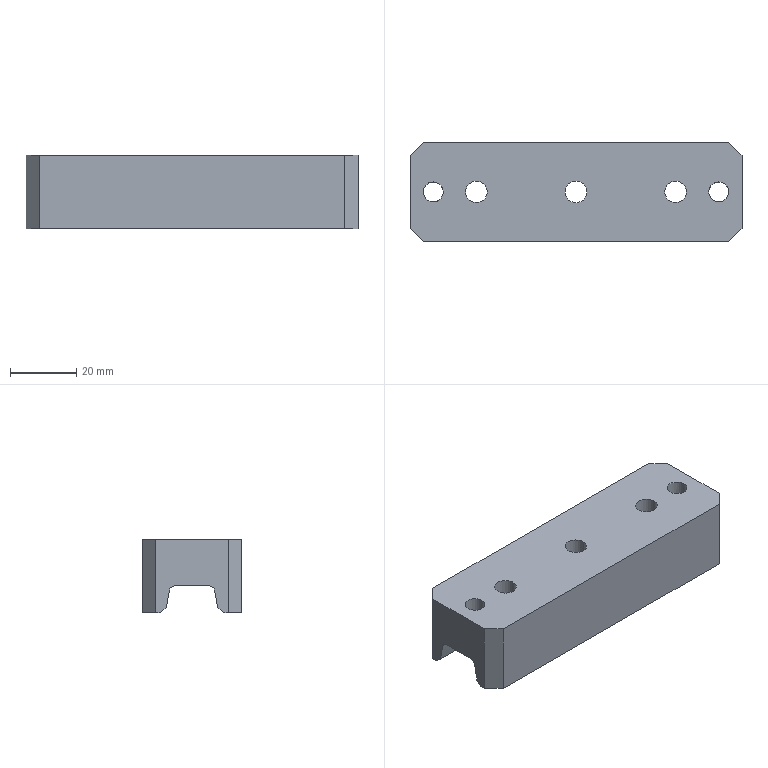Part | STEP file | 车灯-后视镜_id122_x_t | 1 solid | 40 faces | box 100 x 30 x 22 mm | volume 49982 mm3 | plane 26 | cylinder 12 | spline 2 | commonest cylinder face diameters 3 x4 6.5 x3 11 x3 6 x2
STEP:
#1=CARTESIAN_POINT('',(43.,-232.,6.5));
#2=VERTEX_POINT('',#1);
#3=CARTESIAN_POINT('',(43.,-235.,6.5));
#4=DIRECTION('',(0.,0.,-1.));
#5=DIRECTION('',(0.,1.,0.));
#6=AXIS2_PLACEMENT_3D('',#3,#4,#5);
#7=CIRCLE('',#6,3.);
#8=EDGE_CURVE('',#2,#2,#7,.T.);
#9=ORIENTED_EDGE('',*,*,#8,.F.);
#10=EDGE_LOOP('',(#9));
#11=FACE_BOUND('',#10,.T.);
#12=CARTESIAN_POINT('',(50.,-240.331,6.5));
#13=VERTEX_POINT('',#12);
#14=CARTESIAN_POINT('',(31.354,-240.331,6.5));
#15=VERTEX_POINT('',#14);
#16=CARTESIAN_POINT('',(-25.,-240.331,6.5));
#17=DIRECTION('',(-1.,0.,0.));
#18=VECTOR('',#17,1.);
#19=LINE('',#16,#18);
#20=EDGE_CURVE('',#13,#15,#19,.T.);
#21=ORIENTED_EDGE('',*,*,#20,.T.);
#22=CARTESIAN_POINT('',(31.354,-229.669,6.5));
#23=VERTEX_POINT('',#22);
#24=CARTESIAN_POINT('',(30.,-235.,6.5));
#25=DIRECTION('',(0.,0.,1.));
#26=DIRECTION('',(-1.,0.,0.));
#27=AXIS2_PLACEMENT_3D('',#24,#25,#26);
#28=CIRCLE('',#27,5.5);
#29=EDGE_CURVE('',#15,#23,#28,.T.);
#30=ORIENTED_EDGE('',*,*,#29,.T.);
#31=CARTESIAN_POINT('',(50.,-229.669,6.5));
#32=VERTEX_POINT('',#31);
#33=CARTESIAN_POINT('',(0.,-229.669,6.5));
#34=DIRECTION('',(1.,0.,0.));
#35=VECTOR('',#34,1.);
#36=LINE('',#33,#35);
#37=EDGE_CURVE('',#23,#32,#36,.T.);
#38=ORIENTED_EDGE('',*,*,#37,.T.);
#39=CARTESIAN_POINT('',(50.,-317.5,6.5));
#40=DIRECTION('',(0.,1.,0.));
#41=VECTOR('',#40,1.);
#42=LINE('',#39,#41);
#43=EDGE_CURVE('',#13,#32,#42,.T.);
#44=ORIENTED_EDGE('',*,*,#43,.F.);
#45=EDGE_LOOP('',(#21,#30,#38,#44));
#46=FACE_BOUND('',#45,.T.);
#47=CARTESIAN_POINT('',(0.,-317.5,6.5));
#48=DIRECTION('',(0.,0.,1.));
#49=DIRECTION('',(1.,0.,0.));
#50=AXIS2_PLACEMENT_3D('',#47,#48,#49);
#51=PLANE('',#50);
#52=ADVANCED_FACE('',(#11,#46),#51,.F.);
#53=CARTESIAN_POINT('',(-1.354,-240.331,6.5));
#54=VERTEX_POINT('',#53);
#55=CARTESIAN_POINT('',(-28.646,-240.331,6.5));
#56=VERTEX_POINT('',#55);
#57=CARTESIAN_POINT('',(-25.,-240.331,6.5));
#58=DIRECTION('',(-1.,0.,0.));
#59=VECTOR('',#58,1.);
#60=LINE('',#57,#59);
#61=EDGE_CURVE('',#54,#56,#60,.T.);
#62=ORIENTED_EDGE('',*,*,#61,.T.);
#63=CARTESIAN_POINT('',(-28.646,-229.669,6.5));
#64=VERTEX_POINT('',#63);
#65=CARTESIAN_POINT('',(-30.,-235.,6.5));
#66=DIRECTION('',(0.,0.,1.));
#67=DIRECTION('',(-1.,0.,0.));
#68=AXIS2_PLACEMENT_3D('',#65,#66,#67);
#69=CIRCLE('',#68,5.5);
#70=EDGE_CURVE('',#56,#64,#69,.T.);
#71=ORIENTED_EDGE('',*,*,#70,.T.);
#72=CARTESIAN_POINT('',(-1.354,-229.669,6.5));
#73=VERTEX_POINT('',#72);
#74=CARTESIAN_POINT('',(0.,-229.669,6.5));
#75=DIRECTION('',(1.,0.,0.));
#76=VECTOR('',#75,1.);
#77=LINE('',#74,#76);
#78=EDGE_CURVE('',#64,#73,#77,.T.);
#79=ORIENTED_EDGE('',*,*,#78,.T.);
#80=CARTESIAN_POINT('',(0.,-235.,6.5));
#81=DIRECTION('',(0.,0.,-1.));
#82=DIRECTION('',(0.,-1.,0.));
#83=AXIS2_PLACEMENT_3D('',#80,#81,#82);
#84=CIRCLE('',#83,5.5);
#85=EDGE_CURVE('',#54,#73,#84,.T.);
#86=ORIENTED_EDGE('',*,*,#85,.F.);
#87=EDGE_LOOP('',(#62,#71,#79,#86));
#88=FACE_OUTER_BOUND('',#87,.T.);
#89=CARTESIAN_POINT('',(0.,-317.5,6.5));
#90=DIRECTION('',(0.,0.,1.));
#91=DIRECTION('',(1.,0.,0.));
#92=AXIS2_PLACEMENT_3D('',#89,#90,#91);
#93=PLANE('',#92);
#94=ADVANCED_FACE('',(#88),#93,.F.);
#95=CARTESIAN_POINT('',(1.354,-229.669,6.5));
#96=VERTEX_POINT('',#95);
#97=CARTESIAN_POINT('',(28.646,-229.669,6.5));
#98=VERTEX_POINT('',#97);
#99=CARTESIAN_POINT('',(0.,-229.669,6.5));
#100=DIRECTION('',(1.,0.,0.));
#101=VECTOR('',#100,1.);
#102=LINE('',#99,#101);
#103=EDGE_CURVE('',#96,#98,#102,.T.);
#104=ORIENTED_EDGE('',*,*,#103,.T.);
#105=CARTESIAN_POINT('',(28.646,-240.331,6.5));
#106=VERTEX_POINT('',#105);
#107=CARTESIAN_POINT('',(30.,-235.,6.5));
#108=DIRECTION('',(0.,0.,1.));
#109=DIRECTION('',(-1.,0.,0.));
#110=AXIS2_PLACEMENT_3D('',#107,#108,#109);
#111=CIRCLE('',#110,5.5);
#112=EDGE_CURVE('',#98,#106,#111,.T.);
#113=ORIENTED_EDGE('',*,*,#112,.T.);
#114=CARTESIAN_POINT('',(1.354,-240.331,6.5));
#115=VERTEX_POINT('',#114);
#116=CARTESIAN_POINT('',(-25.,-240.331,6.5));
#117=DIRECTION('',(-1.,0.,0.));
#118=VECTOR('',#117,1.);
#119=LINE('',#116,#118);
#120=EDGE_CURVE('',#106,#115,#119,.T.);
#121=ORIENTED_EDGE('',*,*,#120,.T.);
#122=CARTESIAN_POINT('',(0.,-235.,6.5));
#123=DIRECTION('',(0.,0.,-1.));
#124=DIRECTION('',(0.,-1.,0.));
#125=AXIS2_PLACEMENT_3D('',#122,#123,#124);
#126=CIRCLE('',#125,5.5);
#127=EDGE_CURVE('',#96,#115,#126,.T.);
#128=ORIENTED_EDGE('',*,*,#127,.F.);
#129=EDGE_LOOP('',(#104,#113,#121,#128));
#130=FACE_OUTER_BOUND('',#129,.T.);
#131=CARTESIAN_POINT('',(0.,-317.5,6.5));
#132=DIRECTION('',(0.,0.,1.));
#133=DIRECTION('',(1.,0.,0.));
#134=AXIS2_PLACEMENT_3D('',#131,#132,#133);
#135=PLANE('',#134);
#136=ADVANCED_FACE('',(#130),#135,.F.);
#137=CARTESIAN_POINT('',(-43.,-232.,6.5));
#138=VERTEX_POINT('',#137);
#139=CARTESIAN_POINT('',(-43.,-235.,6.5));
#140=DIRECTION('',(0.,0.,-1.));
#141=DIRECTION('',(0.,1.,0.));
#142=AXIS2_PLACEMENT_3D('',#139,#140,#141);
#143=CIRCLE('',#142,3.);
#144=EDGE_CURVE('',#138,#138,#143,.T.);
#145=ORIENTED_EDGE('',*,*,#144,.F.);
#146=EDGE_LOOP('',(#145));
#147=FACE_BOUND('',#146,.T.);
#148=CARTESIAN_POINT('',(-50.,-229.669,6.5));
#149=VERTEX_POINT('',#148);
#150=CARTESIAN_POINT('',(-31.354,-229.669,6.5));
#151=VERTEX_POINT('',#150);
#152=CARTESIAN_POINT('',(0.,-229.669,6.5));
#153=DIRECTION('',(1.,0.,0.));
#154=VECTOR('',#153,1.);
#155=LINE('',#152,#154);
#156=EDGE_CURVE('',#149,#151,#155,.T.);
#157=ORIENTED_EDGE('',*,*,#156,.T.);
#158=CARTESIAN_POINT('',(-31.354,-240.331,6.5));
#159=VERTEX_POINT('',#158);
#160=CARTESIAN_POINT('',(-30.,-235.,6.5));
#161=DIRECTION('',(0.,0.,1.));
#162=DIRECTION('',(-1.,0.,0.));
#163=AXIS2_PLACEMENT_3D('',#160,#161,#162);
#164=CIRCLE('',#163,5.5);
#165=EDGE_CURVE('',#151,#159,#164,.T.);
#166=ORIENTED_EDGE('',*,*,#165,.T.);
#167=CARTESIAN_POINT('',(-50.,-240.331,6.5));
#168=VERTEX_POINT('',#167);
#169=CARTESIAN_POINT('',(-25.,-240.331,6.5));
#170=DIRECTION('',(-1.,0.,0.));
#171=VECTOR('',#170,1.);
#172=LINE('',#169,#171);
#173=EDGE_CURVE('',#159,#168,#172,.T.);
#174=ORIENTED_EDGE('',*,*,#173,.T.);
#175=CARTESIAN_POINT('',(-50.,-317.5,6.5));
#176=DIRECTION('',(0.,-1.,0.));
#177=VECTOR('',#176,1.);
#178=LINE('',#175,#177);
#179=EDGE_CURVE('',#149,#168,#178,.T.);
#180=ORIENTED_EDGE('',*,*,#179,.F.);
#181=EDGE_LOOP('',(#157,#166,#174,#180));
#182=FACE_BOUND('',#181,.T.);
#183=CARTESIAN_POINT('',(0.,-317.5,6.5));
#184=DIRECTION('',(0.,0.,1.));
#185=DIRECTION('',(1.,0.,0.));
#186=AXIS2_PLACEMENT_3D('',#183,#184,#185);
#187=PLANE('',#186);
#188=ADVANCED_FACE('',(#147,#182),#187,.F.);
#189=CARTESIAN_POINT('',(-46.,-235.,20.5));
#190=VERTEX_POINT('',#189);
#191=CARTESIAN_POINT('',(-43.,-235.,20.5));
#192=DIRECTION('',(0.,0.,1.));
#193=DIRECTION('',(-1.,0.,0.));
#194=AXIS2_PLACEMENT_3D('',#191,#192,#193);
#195=CIRCLE('',#194,3.);
#196=EDGE_CURVE('',#190,#190,#195,.T.);
#197=ORIENTED_EDGE('',*,*,#196,.T.);
#198=EDGE_LOOP('',(#197));
#199=FACE_BOUND('',#198,.T.);
#200=ORIENTED_EDGE('',*,*,#144,.T.);
#201=EDGE_LOOP('',(#200));
#202=FACE_BOUND('',#201,.T.);
#203=CARTESIAN_POINT('',(-43.,-235.,40.5));
#204=DIRECTION('',(0.,0.,1.));
#205=DIRECTION('',(1.,0.,0.));
#206=AXIS2_PLACEMENT_3D('',#203,#204,#205);
#207=CYLINDRICAL_SURFACE('',#206,3.);
#208=ADVANCED_FACE('',(#199,#202),#207,.F.);
#209=CARTESIAN_POINT('',(40.,-235.,20.5));
#210=VERTEX_POINT('',#209);
#211=CARTESIAN_POINT('',(43.,-235.,20.5));
#212=DIRECTION('',(0.,0.,1.));
#213=DIRECTION('',(-1.,0.,0.));
#214=AXIS2_PLACEMENT_3D('',#211,#212,#213);
#215=CIRCLE('',#214,3.);
#216=EDGE_CURVE('',#210,#210,#215,.T.);
#217=ORIENTED_EDGE('',*,*,#216,.T.);
#218=EDGE_LOOP('',(#217));
#219=FACE_BOUND('',#218,.T.);
#220=ORIENTED_EDGE('',*,*,#8,.T.);
#221=EDGE_LOOP('',(#220));
#222=FACE_BOUND('',#221,.T.);
#223=CARTESIAN_POINT('',(43.,-235.,40.5));
#224=DIRECTION('',(0.,0.,1.));
#225=DIRECTION('',(1.,0.,0.));
#226=AXIS2_PLACEMENT_3D('',#223,#224,#225);
#227=CYLINDRICAL_SURFACE('',#226,3.);
#228=ADVANCED_FACE('',(#219,#222),#227,.F.);
#229=CARTESIAN_POINT('',(50.,-246.,20.5));
#230=VERTEX_POINT('',#229);
#231=CARTESIAN_POINT('',(50.,-224.,20.5));
#232=VERTEX_POINT('',#231);
#233=CARTESIAN_POINT('',(50.,-317.5,20.5));
#234=DIRECTION('',(0.,1.,0.));
#235=VECTOR('',#234,1.);
#236=LINE('',#233,#235);
#237=EDGE_CURVE('',#230,#232,#236,.T.);
#238=ORIENTED_EDGE('',*,*,#237,.F.);
#239=CARTESIAN_POINT('',(50.,-246.,-1.5));
#240=VERTEX_POINT('',#239);
#241=CARTESIAN_POINT('',(50.,-246.,22.5));
#242=DIRECTION('',(0.,0.,-1.));
#243=VECTOR('',#242,1.);
#244=LINE('',#241,#243);
#245=EDGE_CURVE('',#230,#240,#244,.T.);
#246=ORIENTED_EDGE('',*,*,#245,.T.);
#247=CARTESIAN_POINT('',(50.,-244.5,-1.5));
#248=VERTEX_POINT('',#247);
#249=CARTESIAN_POINT('',(50.,-317.5,-1.5));
#250=DIRECTION('',(0.,1.,0.));
#251=VECTOR('',#250,1.);
#252=LINE('',#249,#251);
#253=EDGE_CURVE('',#240,#248,#252,.T.);
#254=ORIENTED_EDGE('',*,*,#253,.T.);
#255=CARTESIAN_POINT('',(50.,-242.74,-0.02279));
#256=VERTEX_POINT('',#255);
#257=CARTESIAN_POINT('',(50.,-275.52,-27.529));
#258=DIRECTION('',(0.,0.766,0.6428));
#259=VECTOR('',#258,1.);
#260=LINE('',#257,#259);
#261=EDGE_CURVE('',#248,#256,#260,.T.);
#262=ORIENTED_EDGE('',*,*,#261,.T.);
#263=CARTESIAN_POINT('',(50.,-241.808,5.26));
#264=VERTEX_POINT('',#263);
#265=CARTESIAN_POINT('',(50.,-241.142,9.036));
#266=DIRECTION('',(0.,0.1736,0.9848));
#267=VECTOR('',#266,1.);
#268=LINE('',#265,#267);
#269=EDGE_CURVE('',#256,#264,#268,.T.);
#270=ORIENTED_EDGE('',*,*,#269,.T.);
#271=CARTESIAN_POINT('',(50.,-240.331,5.));
#272=DIRECTION('',(-1.,0.,0.));
#273=DIRECTION('',(0.,0.,1.));
#274=AXIS2_PLACEMENT_3D('',#271,#272,#273);
#275=CIRCLE('',#274,1.5);
#276=EDGE_CURVE('',#264,#13,#275,.T.);
#277=ORIENTED_EDGE('',*,*,#276,.T.);
#278=ORIENTED_EDGE('',*,*,#43,.T.);
#279=CARTESIAN_POINT('',(50.,-228.192,5.26));
#280=VERTEX_POINT('',#279);
#281=CARTESIAN_POINT('',(50.,-229.669,5.));
#282=DIRECTION('',(-1.,0.,0.));
#283=DIRECTION('',(0.,0.,1.));
#284=AXIS2_PLACEMENT_3D('',#281,#282,#283);
#285=CIRCLE('',#284,1.5);
#286=EDGE_CURVE('',#32,#280,#285,.T.);
#287=ORIENTED_EDGE('',*,*,#286,.T.);
#288=CARTESIAN_POINT('',(50.,-227.26,-0.02279));
#289=VERTEX_POINT('',#288);
#290=CARTESIAN_POINT('',(50.,-227.,-1.5));
#291=DIRECTION('',(0.,-0.1736,0.9848));
#292=VECTOR('',#291,1.);
#293=LINE('',#290,#292);
#294=EDGE_CURVE('',#289,#280,#293,.T.);
#295=ORIENTED_EDGE('',*,*,#294,.F.);
#296=CARTESIAN_POINT('',(50.,-225.5,-1.5));
#297=VERTEX_POINT('',#296);
#298=CARTESIAN_POINT('',(50.,-291.306,53.717));
#299=DIRECTION('',(0.,0.766,-0.6428));
#300=VECTOR('',#299,1.);
#301=LINE('',#298,#300);
#302=EDGE_CURVE('',#289,#297,#301,.T.);
#303=ORIENTED_EDGE('',*,*,#302,.T.);
#304=CARTESIAN_POINT('',(50.,-224.,-1.5));
#305=VERTEX_POINT('',#304);
#306=CARTESIAN_POINT('',(50.,-317.5,-1.5));
#307=DIRECTION('',(0.,1.,0.));
#308=VECTOR('',#307,1.);
#309=LINE('',#306,#308);
#310=EDGE_CURVE('',#297,#305,#309,.T.);
#311=ORIENTED_EDGE('',*,*,#310,.T.);
#312=CARTESIAN_POINT('',(50.,-224.,22.5));
#313=DIRECTION('',(0.,0.,1.));
#314=VECTOR('',#313,1.);
#315=LINE('',#312,#314);
#316=EDGE_CURVE('',#305,#232,#315,.T.);
#317=ORIENTED_EDGE('',*,*,#316,.T.);
#318=EDGE_LOOP('',(#238,#246,#254,#262,#270,#277,#278,#287,#295,#303,#311,#317));
#319=FACE_OUTER_BOUND('',#318,.T.);
#320=CARTESIAN_POINT('',(50.,-317.5,22.5));
#321=DIRECTION('',(-1.,0.,0.));
#322=DIRECTION('',(0.,0.,1.));
#323=AXIS2_PLACEMENT_3D('',#320,#321,#322);
#324=PLANE('',#323);
#325=ADVANCED_FACE('',(#319),#324,.F.);
#326=CARTESIAN_POINT('',(-50.,-246.,-1.5));
#327=VERTEX_POINT('',#326);
#328=CARTESIAN_POINT('',(-50.,-244.5,-1.5));
#329=VERTEX_POINT('',#328);
#330=CARTESIAN_POINT('',(-50.,-317.5,-1.5));
#331=DIRECTION('',(0.,1.,0.));
#332=VECTOR('',#331,1.);
#333=LINE('',#330,#332);
#334=EDGE_CURVE('',#327,#329,#333,.T.);
#335=ORIENTED_EDGE('',*,*,#334,.F.);
#336=CARTESIAN_POINT('',(-50.,-246.,20.5));
#337=VERTEX_POINT('',#336);
#338=CARTESIAN_POINT('',(-50.,-246.,22.5));
#339=DIRECTION('',(0.,0.,1.));
#340=VECTOR('',#339,1.);
#341=LINE('',#338,#340);
#342=EDGE_CURVE('',#327,#337,#341,.T.);
#343=ORIENTED_EDGE('',*,*,#342,.T.);
#344=CARTESIAN_POINT('',(-50.,-224.,20.5));
#345=VERTEX_POINT('',#344);
#346=CARTESIAN_POINT('',(-50.,-317.5,20.5));
#347=DIRECTION('',(0.,1.,0.));
#348=VECTOR('',#347,1.);
#349=LINE('',#346,#348);
#350=EDGE_CURVE('',#337,#345,#349,.T.);
#351=ORIENTED_EDGE('',*,*,#350,.T.);
#352=CARTESIAN_POINT('',(-50.,-224.,-1.5));
#353=VERTEX_POINT('',#352);
#354=CARTESIAN_POINT('',(-50.,-224.,22.5));
#355=DIRECTION('',(0.,0.,-1.));
#356=VECTOR('',#355,1.);
#357=LINE('',#354,#356);
#358=EDGE_CURVE('',#345,#353,#357,.T.);
#359=ORIENTED_EDGE('',*,*,#358,.T.);
#360=CARTESIAN_POINT('',(-50.,-225.5,-1.5));
#361=VERTEX_POINT('',#360);
#362=CARTESIAN_POINT('',(-50.,-317.5,-1.5));
#363=DIRECTION('',(0.,1.,0.));
#364=VECTOR('',#363,1.);
#365=LINE('',#362,#364);
#366=EDGE_CURVE('',#361,#353,#365,.T.);
#367=ORIENTED_EDGE('',*,*,#366,.F.);
#368=CARTESIAN_POINT('',(-50.,-227.26,-0.02279));
#369=VERTEX_POINT('',#368);
#370=CARTESIAN_POINT('',(-50.,-291.306,53.717));
#371=DIRECTION('',(0.,-0.766,0.6428));
#372=VECTOR('',#371,1.);
#373=LINE('',#370,#372);
#374=EDGE_CURVE('',#361,#369,#373,.T.);
#375=ORIENTED_EDGE('',*,*,#374,.T.);
#376=CARTESIAN_POINT('',(-50.,-228.192,5.26));
#377=VERTEX_POINT('',#376);
#378=CARTESIAN_POINT('',(-50.,-233.833,37.253));
#379=DIRECTION('',(0.,-0.1736,0.9848));
#380=VECTOR('',#379,1.);
#381=LINE('',#378,#380);
#382=EDGE_CURVE('',#369,#377,#381,.T.);
#383=ORIENTED_EDGE('',*,*,#382,.T.);
#384=CARTESIAN_POINT('',(-50.,-229.669,5.));
#385=DIRECTION('',(1.,0.,0.));
#386=DIRECTION('',(0.,0.,1.));
#387=AXIS2_PLACEMENT_3D('',#384,#385,#386);
#388=CIRCLE('',#387,1.5);
#389=EDGE_CURVE('',#377,#149,#388,.T.);
#390=ORIENTED_EDGE('',*,*,#389,.T.);
#391=ORIENTED_EDGE('',*,*,#179,.T.);
#392=CARTESIAN_POINT('',(-50.,-241.808,5.26));
#393=VERTEX_POINT('',#392);
#394=CARTESIAN_POINT('',(-50.,-240.331,5.));
#395=DIRECTION('',(1.,0.,0.));
#396=DIRECTION('',(0.,0.,1.));
#397=AXIS2_PLACEMENT_3D('',#394,#395,#396);
#398=CIRCLE('',#397,1.5);
#399=EDGE_CURVE('',#168,#393,#398,.T.);
#400=ORIENTED_EDGE('',*,*,#399,.T.);
#401=CARTESIAN_POINT('',(-50.,-242.74,-0.02279));
#402=VERTEX_POINT('',#401);
#403=CARTESIAN_POINT('',(-50.,-243.,-1.5));
#404=DIRECTION('',(0.,0.1736,0.9848));
#405=VECTOR('',#404,1.);
#406=LINE('',#403,#405);
#407=EDGE_CURVE('',#402,#393,#406,.T.);
#408=ORIENTED_EDGE('',*,*,#407,.F.);
#409=CARTESIAN_POINT('',(-50.,-275.52,-27.529));
#410=DIRECTION('',(0.,-0.766,-0.6428));
#411=VECTOR('',#410,1.);
#412=LINE('',#409,#411);
#413=EDGE_CURVE('',#402,#329,#412,.T.);
#414=ORIENTED_EDGE('',*,*,#413,.T.);
#415=EDGE_LOOP('',(#335,#343,#351,#359,#367,#375,#383,#390,#391,#400,#408,#414));
#416=FACE_OUTER_BOUND('',#415,.T.);
#417=CARTESIAN_POINT('',(-50.,-317.5,22.5));
#418=DIRECTION('',(-1.,0.,0.));
#419=DIRECTION('',(0.,0.,1.));
#420=AXIS2_PLACEMENT_3D('',#417,#418,#419);
#421=PLANE('',#420);
#422=ADVANCED_FACE('',(#416),#421,.T.);
#423=CARTESIAN_POINT('',(46.,-220.,20.5));
#424=VERTEX_POINT('',#423);
#425=CARTESIAN_POINT('',(-46.,-220.,20.5));
#426=VERTEX_POINT('',#425);
#427=CARTESIAN_POINT('',(0.,-220.,20.5));
#428=DIRECTION('',(-1.,0.,0.));
#429=VECTOR('',#428,1.);
#430=LINE('',#427,#429);
#431=EDGE_CURVE('',#424,#426,#430,.T.);
#432=ORIENTED_EDGE('',*,*,#431,.F.);
#433=CARTESIAN_POINT('',(46.,-220.,-1.5));
#434=VERTEX_POINT('',#433);
#435=CARTESIAN_POINT('',(46.,-220.,22.5));
#436=DIRECTION('',(0.,0.,-1.));
#437=VECTOR('',#436,1.);
#438=LINE('',#435,#437);
#439=EDGE_CURVE('',#424,#434,#438,.T.);
#440=ORIENTED_EDGE('',*,*,#439,.T.);
#441=CARTESIAN_POINT('',(-46.,-220.,-1.5));
#442=VERTEX_POINT('',#441);
#443=CARTESIAN_POINT('',(0.,-220.,-1.5));
#444=DIRECTION('',(-1.,0.,0.));
#445=VECTOR('',#444,1.);
#446=LINE('',#443,#445);
#447=EDGE_CURVE('',#434,#442,#446,.T.);
#448=ORIENTED_EDGE('',*,*,#447,.T.);
#449=CARTESIAN_POINT('',(-46.,-220.,20.5));
#450=DIRECTION('',(0.,0.,1.));
#451=VECTOR('',#450,1.);
#452=LINE('',#449,#451);
#453=EDGE_CURVE('',#442,#426,#452,.T.);
#454=ORIENTED_EDGE('',*,*,#453,.T.);
#455=EDGE_LOOP('',(#432,#440,#448,#454));
#456=FACE_OUTER_BOUND('',#455,.T.);
#457=CARTESIAN_POINT('',(0.,-220.,22.5));
#458=DIRECTION('',(0.,-1.,0.));
#459=DIRECTION('',(0.,0.,-1.));
#460=AXIS2_PLACEMENT_3D('',#457,#458,#459);
#461=PLANE('',#460);
#462=ADVANCED_FACE('',(#456),#461,.F.);
#463=CARTESIAN_POINT('',(46.,-250.,20.5));
#464=VERTEX_POINT('',#463);
#465=CARTESIAN_POINT('',(-46.,-250.,20.5));
#466=VERTEX_POINT('',#465);
#467=CARTESIAN_POINT('',(0.,-250.,20.5));
#468=DIRECTION('',(-1.,0.,0.));
#469=VECTOR('',#468,1.);
#470=LINE('',#467,#469);
#471=EDGE_CURVE('',#464,#466,#470,.T.);
#472=ORIENTED_EDGE('',*,*,#471,.T.);
#473=CARTESIAN_POINT('',(-46.,-250.,-1.5));
#474=VERTEX_POINT('',#473);
#475=CARTESIAN_POINT('',(-46.,-250.,22.5));
#476=DIRECTION('',(0.,0.,-1.));
#477=VECTOR('',#476,1.);
#478=LINE('',#475,#477);
#479=EDGE_CURVE('',#466,#474,#478,.T.);
#480=ORIENTED_EDGE('',*,*,#479,.T.);
#481=CARTESIAN_POINT('',(46.,-250.,-1.5));
#482=VERTEX_POINT('',#481);
#483=CARTESIAN_POINT('',(0.,-250.,-1.5));
#484=DIRECTION('',(-1.,0.,0.));
#485=VECTOR('',#484,1.);
#486=LINE('',#483,#485);
#487=EDGE_CURVE('',#482,#474,#486,.T.);
#488=ORIENTED_EDGE('',*,*,#487,.F.);
#489=CARTESIAN_POINT('',(46.,-250.,20.5));
#490=DIRECTION('',(0.,0.,1.));
#491=VECTOR('',#490,1.);
#492=LINE('',#489,#491);
#493=EDGE_CURVE('',#482,#464,#492,.T.);
#494=ORIENTED_EDGE('',*,*,#493,.T.);
#495=EDGE_LOOP('',(#472,#480,#488,#494));
#496=FACE_OUTER_BOUND('',#495,.T.);
#497=CARTESIAN_POINT('',(0.,-250.,22.5));
#498=DIRECTION('',(0.,-1.,0.));
#499=DIRECTION('',(0.,0.,-1.));
#500=AXIS2_PLACEMENT_3D('',#497,#498,#499);
#501=PLANE('',#500);
#502=ADVANCED_FACE('',(#496),#501,.T.);
#503=CARTESIAN_POINT('',(30.,-238.25,20.5));
#504=VERTEX_POINT('',#503);
#505=CARTESIAN_POINT('',(30.,-235.,20.5));
#506=DIRECTION('',(0.,0.,1.));
#507=DIRECTION('',(0.,-1.,0.));
#508=AXIS2_PLACEMENT_3D('',#505,#506,#507);
#509=CIRCLE('',#508,3.25);
#510=EDGE_CURVE('',#504,#504,#509,.T.);
#511=ORIENTED_EDGE('',*,*,#510,.F.);
#512=EDGE_LOOP('',(#511));
#513=FACE_BOUND('',#512,.T.);
#514=CARTESIAN_POINT('',(-30.,-238.25,20.5));
#515=VERTEX_POINT('',#514);
#516=CARTESIAN_POINT('',(-30.,-235.,20.5));
#517=DIRECTION('',(0.,0.,1.));
#518=DIRECTION('',(0.,-1.,0.));
#519=AXIS2_PLACEMENT_3D('',#516,#517,#518);
#520=CIRCLE('',#519,3.25);
#521=EDGE_CURVE('',#515,#515,#520,.T.);
#522=ORIENTED_EDGE('',*,*,#521,.F.);
#523=EDGE_LOOP('',(#522));
#524=FACE_BOUND('',#523,.T.);
#525=ORIENTED_EDGE('',*,*,#216,.F.);
#526=EDGE_LOOP('',(#525));
#527=FACE_BOUND('',#526,.T.);
#528=ORIENTED_EDGE('',*,*,#196,.F.);
#529=EDGE_LOOP('',(#528));
#530=FACE_BOUND('',#529,.T.);
#531=CARTESIAN_POINT('',(0.,-238.25,20.5));
#532=VERTEX_POINT('',#531);
#533=CARTESIAN_POINT('',(0.,-235.,20.5));
#534=DIRECTION('',(0.,0.,1.));
#535=DIRECTION('',(0.,-1.,0.));
#536=AXIS2_PLACEMENT_3D('',#533,#534,#535);
#537=CIRCLE('',#536,3.25);
#538=EDGE_CURVE('',#532,#532,#537,.T.);
#539=ORIENTED_EDGE('',*,*,#538,.F.);
#540=EDGE_LOOP('',(#539));
#541=FACE_BOUND('',#540,.T.);
#542=ORIENTED_EDGE('',*,*,#350,.F.);
#543=CARTESIAN_POINT('',(10.75,-306.75,20.5));
#544=DIRECTION('',(0.7071,-0.7071,0.));
#545=VECTOR('',#544,1.);
#546=LINE('',#543,#545);
#547=EDGE_CURVE('',#337,#466,#546,.T.);
#548=ORIENTED_EDGE('',*,*,#547,.T.);
#549=ORIENTED_EDGE('',*,*,#471,.F.);
#550=CARTESIAN_POINT('',(-10.75,-306.75,20.5));
#551=DIRECTION('',(0.7071,0.7071,0.));
#552=VECTOR('',#551,1.);
#553=LINE('',#550,#552);
#554=EDGE_CURVE('',#464,#230,#553,.T.);
#555=ORIENTED_EDGE('',*,*,#554,.T.);
#556=ORIENTED_EDGE('',*,*,#237,.T.);
#557=CARTESIAN_POINT('',(71.75,-245.75,20.5));
#558=DIRECTION('',(-0.7071,0.7071,0.));
#559=VECTOR('',#558,1.);
#560=LINE('',#557,#559);
#561=EDGE_CURVE('',#232,#424,#560,.T.);
#562=ORIENTED_EDGE('',*,*,#561,.T.);
#563=ORIENTED_EDGE('',*,*,#431,.T.);
#564=CARTESIAN_POINT('',(-71.75,-245.75,20.5));
#565=DIRECTION('',(-0.7071,-0.7071,0.));
#566=VECTOR('',#565,1.);
#567=LINE('',#564,#566);
#568=EDGE_CURVE('',#426,#345,#567,.T.);
#569=ORIENTED_EDGE('',*,*,#568,.T.);
#570=EDGE_LOOP('',(#542,#548,#549,#555,#556,#562,#563,#569));
#571=FACE_BOUND('',#570,.T.);
#572=CARTESIAN_POINT('',(0.,-317.5,20.5));
#573=DIRECTION('',(0.,0.,1.));
#574=DIRECTION('',(1.,0.,0.));
#575=AXIS2_PLACEMENT_3D('',#572,#573,#574);
#576=PLANE('',#575);
#577=ADVANCED_FACE('',(#513,#524,#527,#530,#541,#571),#576,.T.);
#578=CARTESIAN_POINT('',(0.,-231.75,13.5));
#579=VERTEX_POINT('',#578);
#580=CARTESIAN_POINT('',(0.,-235.,13.5));
#581=DIRECTION('',(0.,0.,-1.));
#582=DIRECTION('',(0.,1.,0.));
#583=AXIS2_PLACEMENT_3D('',#580,#581,#582);
#584=CIRCLE('',#583,3.25);
#585=EDGE_CURVE('',#579,#579,#584,.T.);
#586=ORIENTED_EDGE('',*,*,#585,.T.);
#587=EDGE_LOOP('',(#586));
#588=FACE_BOUND('',#587,.T.);
#589=ORIENTED_EDGE('',*,*,#538,.T.);
#590=EDGE_LOOP('',(#589));
#591=FACE_BOUND('',#590,.T.);
#592=CARTESIAN_POINT('',(0.,-235.,10.5));
#593=DIRECTION('',(0.,0.,1.));
#594=DIRECTION('',(1.,0.,0.));
#595=AXIS2_PLACEMENT_3D('',#592,#593,#594);
#596=CYLINDRICAL_SURFACE('',#595,3.25);
#597=ADVANCED_FACE('',(#588,#591),#596,.F.);
#598=CARTESIAN_POINT('',(0.,-240.5,13.5));
#599=VERTEX_POINT('',#598);
#600=CARTESIAN_POINT('',(0.,-235.,13.5));
#601=DIRECTION('',(0.,0.,-1.));
#602=DIRECTION('',(0.,-1.,0.));
#603=AXIS2_PLACEMENT_3D('',#600,#601,#602);
#604=CIRCLE('',#603,5.5);
#605=EDGE_CURVE('',#599,#599,#604,.T.);
#606=ORIENTED_EDGE('',*,*,#605,.T.);
#607=EDGE_LOOP('',(#606));
#608=FACE_BOUND('',#607,.T.);
#609=ORIENTED_EDGE('',*,*,#585,.F.);
#610=EDGE_LOOP('',(#609));
#611=FACE_BOUND('',#610,.T.);
#612=CARTESIAN_POINT('',(0.,-235.,13.5));
#613=DIRECTION('',(0.,0.,1.));
#614=DIRECTION('',(0.,-1.,0.));
#615=AXIS2_PLACEMENT_3D('',#612,#613,#614);
#616=PLANE('',#615);
#617=ADVANCED_FACE('',(#608,#611),#616,.F.);
#618=ORIENTED_EDGE('',*,*,#85,.T.);
#619=CARTESIAN_POINT('',(0.,-235.,6.5));
#620=DIRECTION('',(0.,0.,-1.));
#621=DIRECTION('',(0.,-1.,0.));
#622=AXIS2_PLACEMENT_3D('',#619,#620,#621);
#623=CIRCLE('',#622,5.5);
#624=EDGE_CURVE('',#73,#96,#623,.T.);
#625=ORIENTED_EDGE('',*,*,#624,.T.);
#626=ORIENTED_EDGE('',*,*,#127,.T.);
#627=CARTESIAN_POINT('',(0.,-235.,6.5));
#628=DIRECTION('',(0.,0.,-1.));
#629=DIRECTION('',(0.,-1.,0.));
#630=AXIS2_PLACEMENT_3D('',#627,#628,#629);
#631=CIRCLE('',#630,5.5);
#632=EDGE_CURVE('',#115,#54,#631,.T.);
#633=ORIENTED_EDGE('',*,*,#632,.T.);
#634=EDGE_LOOP('',(#618,#625,#626,#633));
#635=FACE_BOUND('',#634,.T.);
#636=ORIENTED_EDGE('',*,*,#605,.F.);
#637=EDGE_LOOP('',(#636));
#638=FACE_BOUND('',#637,.T.);
#639=CARTESIAN_POINT('',(0.,-235.,6.));
#640=DIRECTION('',(0.,0.,1.));
#641=DIRECTION('',(0.,-1.,0.));
#642=AXIS2_PLACEMENT_3D('',#639,#640,#641);
#643=CYLINDRICAL_SURFACE('',#642,5.5);
#644=ADVANCED_FACE('',(#635,#638),#643,.F.);
#645=ORIENTED_EDGE('',*,*,#487,.T.);
#646=CARTESIAN_POINT('',(10.75,-306.75,-1.5));
#647=DIRECTION('',(-0.7071,0.7071,0.));
#648=VECTOR('',#647,1.);
#649=LINE('',#646,#648);
#650=EDGE_CURVE('',#474,#327,#649,.T.);
#651=ORIENTED_EDGE('',*,*,#650,.T.);
#652=ORIENTED_EDGE('',*,*,#334,.T.);
#653=CARTESIAN_POINT('',(0.,-244.5,-1.5));
#654=DIRECTION('',(1.,0.,0.));
#655=VECTOR('',#654,1.);
#656=LINE('',#653,#655);
#657=EDGE_CURVE('',#329,#248,#656,.T.);
#658=ORIENTED_EDGE('',*,*,#657,.T.);
#659=ORIENTED_EDGE('',*,*,#253,.F.);
#660=CARTESIAN_POINT('',(-10.75,-306.75,-1.5));
#661=DIRECTION('',(-0.7071,-0.7071,0.));
#662=VECTOR('',#661,1.);
#663=LINE('',#660,#662);
#664=EDGE_CURVE('',#240,#482,#663,.T.);
#665=ORIENTED_EDGE('',*,*,#664,.T.);
#666=EDGE_LOOP('',(#645,#651,#652,#658,#659,#665));
#667=FACE_OUTER_BOUND('',#666,.T.);
#668=CARTESIAN_POINT('',(0.,-317.5,-1.5));
#669=DIRECTION('',(0.,0.,1.));
#670=DIRECTION('',(1.,0.,0.));
#671=AXIS2_PLACEMENT_3D('',#668,#669,#670);
#672=PLANE('',#671);
#673=ADVANCED_FACE('',(#667),#672,.F.);
#674=ORIENTED_EDGE('',*,*,#407,.T.);
#675=CARTESIAN_POINT('',(-1.354,-241.808,5.26));
#676=VERTEX_POINT('',#675);
#677=CARTESIAN_POINT('',(25.,-241.808,5.26));
#678=DIRECTION('',(1.,0.,0.));
#679=VECTOR('',#678,1.);
#680=LINE('',#677,#679);
#681=EDGE_CURVE('',#393,#676,#680,.T.);
#682=ORIENTED_EDGE('',*,*,#681,.T.);
#683=CARTESIAN_POINT('',(1.354,-241.808,5.26));
#684=VERTEX_POINT('',#683);
#685=CARTESIAN_POINT('',(-1.354,-241.808,5.26));
#686=CARTESIAN_POINT('',(-0.9026,-241.808,5.26));
#687=CARTESIAN_POINT('',(-0.4513,-241.806,5.27));
#688=CARTESIAN_POINT('',(0.,-241.806,5.27));
#689=CARTESIAN_POINT('',(0.4513,-241.806,5.27));
#690=CARTESIAN_POINT('',(0.9026,-241.808,5.26));
#691=CARTESIAN_POINT('',(1.354,-241.808,5.26));
#692=B_SPLINE_CURVE_WITH_KNOTS('',3,(#685,#686,#687,#688,#689,#690,#691),.UNSPECIFIED.,.F.,.F.,(4,3,4),(0.,0.5,1.),.UNSPECIFIED.);
#693=EDGE_CURVE('',#676,#684,#692,.T.);
#694=ORIENTED_EDGE('',*,*,#693,.T.);
#695=CARTESIAN_POINT('',(25.,-241.808,5.26));
#696=DIRECTION('',(1.,0.,0.));
#697=VECTOR('',#696,1.);
#698=LINE('',#695,#697);
#699=EDGE_CURVE('',#684,#264,#698,.T.);
#700=ORIENTED_EDGE('',*,*,#699,.T.);
#701=ORIENTED_EDGE('',*,*,#269,.F.);
#702=CARTESIAN_POINT('',(25.,-242.74,-0.02279));
#703=DIRECTION('',(-1.,0.,0.));
#704=VECTOR('',#703,1.);
#705=LINE('',#702,#704);
#706=EDGE_CURVE('',#256,#402,#705,.T.);
#707=ORIENTED_EDGE('',*,*,#706,.T.);
#708=EDGE_LOOP('',(#674,#682,#694,#700,#701,#707));
#709=FACE_OUTER_BOUND('',#708,.T.);
#710=CARTESIAN_POINT('',(25.,-243.,-1.5));
#711=DIRECTION('',(0.,0.9848,-0.1736));
#712=DIRECTION('',(0.,0.1736,0.9848));
#713=AXIS2_PLACEMENT_3D('',#710,#711,#712);
#714=PLANE('',#713);
#715=ADVANCED_FACE('',(#709),#714,.T.);
#716=ORIENTED_EDGE('',*,*,#447,.F.);
#717=CARTESIAN_POINT('',(71.75,-245.75,-1.5));
#718=DIRECTION('',(0.7071,-0.7071,0.));
#719=VECTOR('',#718,1.);
#720=LINE('',#717,#719);
#721=EDGE_CURVE('',#434,#305,#720,.T.);
#722=ORIENTED_EDGE('',*,*,#721,.T.);
#723=ORIENTED_EDGE('',*,*,#310,.F.);
#724=CARTESIAN_POINT('',(-25.,-225.5,-1.5));
#725=DIRECTION('',(-1.,0.,0.));
#726=VECTOR('',#725,1.);
#727=LINE('',#724,#726);
#728=EDGE_CURVE('',#297,#361,#727,.T.);
#729=ORIENTED_EDGE('',*,*,#728,.T.);
#730=ORIENTED_EDGE('',*,*,#366,.T.);
#731=CARTESIAN_POINT('',(-71.75,-245.75,-1.5));
#732=DIRECTION('',(0.7071,0.7071,0.));
#733=VECTOR('',#732,1.);
#734=LINE('',#731,#733);
#735=EDGE_CURVE('',#353,#442,#734,.T.);
#736=ORIENTED_EDGE('',*,*,#735,.T.);
#737=EDGE_LOOP('',(#716,#722,#723,#729,#730,#736));
#738=FACE_OUTER_BOUND('',#737,.T.);
#739=CARTESIAN_POINT('',(0.,-317.5,-1.5));
#740=DIRECTION('',(0.,0.,1.));
#741=DIRECTION('',(1.,0.,0.));
#742=AXIS2_PLACEMENT_3D('',#739,#740,#741);
#743=PLANE('',#742);
#744=ADVANCED_FACE('',(#738),#743,.F.);
#745=ORIENTED_EDGE('',*,*,#294,.T.);
#746=CARTESIAN_POINT('',(1.354,-228.192,5.26));
#747=VERTEX_POINT('',#746);
#748=CARTESIAN_POINT('',(25.,-228.192,5.26));
#749=DIRECTION('',(-1.,0.,0.));
#750=VECTOR('',#749,1.);
#751=LINE('',#748,#750);
#752=EDGE_CURVE('',#280,#747,#751,.T.);
#753=ORIENTED_EDGE('',*,*,#752,.T.);
#754=CARTESIAN_POINT('',(-1.354,-228.192,5.26));
#755=VERTEX_POINT('',#754);
#756=CARTESIAN_POINT('',(1.354,-228.192,5.26));
#757=CARTESIAN_POINT('',(0.9026,-228.192,5.26));
#758=CARTESIAN_POINT('',(0.4513,-228.194,5.27));
#759=CARTESIAN_POINT('',(0.,-228.194,5.27));
#760=CARTESIAN_POINT('',(-0.4513,-228.194,5.27));
#761=CARTESIAN_POINT('',(-0.9026,-228.192,5.26));
#762=CARTESIAN_POINT('',(-1.354,-228.192,5.26));
#763=B_SPLINE_CURVE_WITH_KNOTS('',3,(#756,#757,#758,#759,#760,#761,#762),.UNSPECIFIED.,.F.,.F.,(4,3,4),(0.,0.5,1.),.UNSPECIFIED.);
#764=EDGE_CURVE('',#747,#755,#763,.T.);
#765=ORIENTED_EDGE('',*,*,#764,.T.);
#766=CARTESIAN_POINT('',(25.,-228.192,5.26));
#767=DIRECTION('',(-1.,0.,0.));
#768=VECTOR('',#767,1.);
#769=LINE('',#766,#768);
#770=EDGE_CURVE('',#755,#377,#769,.T.);
#771=ORIENTED_EDGE('',*,*,#770,.T.);
#772=ORIENTED_EDGE('',*,*,#382,.F.);
#773=CARTESIAN_POINT('',(25.,-227.26,-0.02279));
#774=DIRECTION('',(1.,0.,0.));
#775=VECTOR('',#774,1.);
#776=LINE('',#773,#775);
#777=EDGE_CURVE('',#369,#289,#776,.T.);
#778=ORIENTED_EDGE('',*,*,#777,.T.);
#779=EDGE_LOOP('',(#745,#753,#765,#771,#772,#778));
#780=FACE_OUTER_BOUND('',#779,.T.);
#781=CARTESIAN_POINT('',(25.,-227.,-1.5));
#782=DIRECTION('',(0.,-0.9848,-0.1736));
#783=DIRECTION('',(0.,0.1736,-0.9848));
#784=AXIS2_PLACEMENT_3D('',#781,#782,#783);
#785=PLANE('',#784);
#786=ADVANCED_FACE('',(#780),#785,.T.);
#787=ORIENTED_EDGE('',*,*,#413,.F.);
#788=ORIENTED_EDGE('',*,*,#706,.F.);
#789=ORIENTED_EDGE('',*,*,#261,.F.);
#790=ORIENTED_EDGE('',*,*,#657,.F.);
#791=EDGE_LOOP('',(#787,#788,#789,#790));
#792=FACE_OUTER_BOUND('',#791,.T.);
#793=CARTESIAN_POINT('',(0.,-244.5,-1.5));
#794=DIRECTION('',(0.,0.6428,-0.766));
#795=DIRECTION('',(0.,0.766,0.6428));
#796=AXIS2_PLACEMENT_3D('',#793,#794,#795);
#797=PLANE('',#796);
#798=ADVANCED_FACE('',(#792),#797,.T.);
#799=ORIENTED_EDGE('',*,*,#374,.F.);
#800=ORIENTED_EDGE('',*,*,#728,.F.);
#801=ORIENTED_EDGE('',*,*,#302,.F.);
#802=ORIENTED_EDGE('',*,*,#777,.F.);
#803=EDGE_LOOP('',(#799,#800,#801,#802));
#804=FACE_OUTER_BOUND('',#803,.T.);
#805=CARTESIAN_POINT('',(25.,-227.26,-0.02279));
#806=DIRECTION('',(0.,-0.6428,-0.766));
#807=DIRECTION('',(0.,0.766,-0.6428));
#808=AXIS2_PLACEMENT_3D('',#805,#806,#807);
#809=PLANE('',#808);
#810=ADVANCED_FACE('',(#804),#809,.T.);
#811=ORIENTED_EDGE('',*,*,#276,.F.);
#812=ORIENTED_EDGE('',*,*,#699,.F.);
#813=CARTESIAN_POINT('',(1.354,-240.331,5.));
#814=DIRECTION('',(1.,0.,0.));
#815=DIRECTION('',(0.,0.,1.));
#816=AXIS2_PLACEMENT_3D('',#813,#814,#815);
#817=CIRCLE('',#816,1.5);
#818=EDGE_CURVE('',#115,#684,#817,.T.);
#819=ORIENTED_EDGE('',*,*,#818,.F.);
#820=ORIENTED_EDGE('',*,*,#120,.F.);
#821=CARTESIAN_POINT('',(25.,-240.331,6.5));
#822=DIRECTION('',(-1.,0.,0.));
#823=VECTOR('',#822,1.);
#824=LINE('',#821,#823);
#825=EDGE_CURVE('',#15,#106,#824,.T.);
#826=ORIENTED_EDGE('',*,*,#825,.F.);
#827=ORIENTED_EDGE('',*,*,#20,.F.);
#828=EDGE_LOOP('',(#811,#812,#819,#820,#826,#827));
#829=FACE_OUTER_BOUND('',#828,.T.);
#830=CARTESIAN_POINT('',(25.,-240.331,5.));
#831=DIRECTION('',(1.,0.,0.));
#832=DIRECTION('',(0.,0.,1.));
#833=AXIS2_PLACEMENT_3D('',#830,#831,#832);
#834=CYLINDRICAL_SURFACE('',#833,1.5);
#835=ADVANCED_FACE('',(#829),#834,.F.);
#836=ORIENTED_EDGE('',*,*,#818,.T.);
#837=ORIENTED_EDGE('',*,*,#693,.F.);
#838=CARTESIAN_POINT('',(-1.354,-240.331,5.));
#839=DIRECTION('',(1.,0.,0.));
#840=DIRECTION('',(0.,0.,-1.));
#841=AXIS2_PLACEMENT_3D('',#838,#839,#840);
#842=CIRCLE('',#841,1.5);
#843=EDGE_CURVE('',#54,#676,#842,.T.);
#844=ORIENTED_EDGE('',*,*,#843,.F.);
#845=ORIENTED_EDGE('',*,*,#632,.F.);
#846=EDGE_LOOP('',(#836,#837,#844,#845));
#847=FACE_OUTER_BOUND('',#846,.T.);
#848=CARTESIAN_POINT('',(1.354,-241.808,5.26));
#849=CARTESIAN_POINT('',(1.354,-241.589,6.5));
#850=CARTESIAN_POINT('',(1.354,-240.331,6.5));
#851=CARTESIAN_POINT('',(0.4512,-241.808,5.26));
#852=CARTESIAN_POINT('',(0.5565,-241.619,6.332));
#853=CARTESIAN_POINT('',(0.4966,-240.549,6.5));
#854=CARTESIAN_POINT('',(-0.4514,-241.808,5.26));
#855=CARTESIAN_POINT('',(-0.5567,-241.619,6.332));
#856=CARTESIAN_POINT('',(-0.4968,-240.548,6.5));
#857=CARTESIAN_POINT('',(-1.354,-241.808,5.26));
#858=CARTESIAN_POINT('',(-1.354,-241.589,6.5));
#859=CARTESIAN_POINT('',(-1.354,-240.331,6.5));
#860=(BOUNDED_SURFACE()B_SPLINE_SURFACE(3,2,((#848,#849,#850),(#851,#852,#853),(#854,#855,#856),(#857,#858,#859)),.UNSPECIFIED.,.F.,.F.,.F.)B_SPLINE_SURFACE_WITH_KNOTS((4,4),(3,3),(0.,1.),(0.,1.),.UNSPECIFIED.)GEOMETRIC_REPRESENTATION_ITEM()RATIONAL_B_SPLINE_SURFACE(((1.,0.766,1.),(1.,0.8131,1.),(1.,0.8131,1.),(1.,0.766,1.)))REPRESENTATION_ITEM('')SURFACE());
#861=ADVANCED_FACE('',(#847),#860,.T.);
#862=ORIENTED_EDGE('',*,*,#399,.F.);
#863=ORIENTED_EDGE('',*,*,#173,.F.);
#864=CARTESIAN_POINT('',(25.,-240.331,6.5));
#865=DIRECTION('',(-1.,0.,0.));
#866=VECTOR('',#865,1.);
#867=LINE('',#864,#866);
#868=EDGE_CURVE('',#56,#159,#867,.T.);
#869=ORIENTED_EDGE('',*,*,#868,.F.);
#870=ORIENTED_EDGE('',*,*,#61,.F.);
#871=ORIENTED_EDGE('',*,*,#843,.T.);
#872=ORIENTED_EDGE('',*,*,#681,.F.);
#873=EDGE_LOOP('',(#862,#863,#869,#870,#871,#872));
#874=FACE_OUTER_BOUND('',#873,.T.);
#875=CARTESIAN_POINT('',(25.,-240.331,5.));
#876=DIRECTION('',(1.,0.,0.));
#877=DIRECTION('',(0.,0.,1.));
#878=AXIS2_PLACEMENT_3D('',#875,#876,#877);
#879=CYLINDRICAL_SURFACE('',#878,1.5);
#880=ADVANCED_FACE('',(#874),#879,.F.);
#881=ORIENTED_EDGE('',*,*,#286,.F.);
#882=ORIENTED_EDGE('',*,*,#37,.F.);
#883=CARTESIAN_POINT('',(0.,-229.669,6.5));
#884=DIRECTION('',(1.,0.,0.));
#885=VECTOR('',#884,1.);
#886=LINE('',#883,#885);
#887=EDGE_CURVE('',#98,#23,#886,.T.);
#888=ORIENTED_EDGE('',*,*,#887,.F.);
#889=ORIENTED_EDGE('',*,*,#103,.F.);
#890=CARTESIAN_POINT('',(1.354,-229.669,5.));
#891=DIRECTION('',(1.,0.,0.));
#892=DIRECTION('',(0.,0.,1.));
#893=AXIS2_PLACEMENT_3D('',#890,#891,#892);
#894=CIRCLE('',#893,1.5);
#895=EDGE_CURVE('',#747,#96,#894,.T.);
#896=ORIENTED_EDGE('',*,*,#895,.F.);
#897=ORIENTED_EDGE('',*,*,#752,.F.);
#898=EDGE_LOOP('',(#881,#882,#888,#889,#896,#897));
#899=FACE_OUTER_BOUND('',#898,.T.);
#900=CARTESIAN_POINT('',(0.,-229.669,5.));
#901=DIRECTION('',(1.,0.,0.));
#902=DIRECTION('',(0.,0.,1.));
#903=AXIS2_PLACEMENT_3D('',#900,#901,#902);
#904=CYLINDRICAL_SURFACE('',#903,1.5);
#905=ADVANCED_FACE('',(#899),#904,.F.);
#906=ORIENTED_EDGE('',*,*,#895,.T.);
#907=ORIENTED_EDGE('',*,*,#624,.F.);
#908=CARTESIAN_POINT('',(-1.354,-229.669,5.));
#909=DIRECTION('',(1.,0.,0.));
#910=DIRECTION('',(0.,0.,1.));
#911=AXIS2_PLACEMENT_3D('',#908,#909,#910);
#912=CIRCLE('',#911,1.5);
#913=EDGE_CURVE('',#755,#73,#912,.T.);
#914=ORIENTED_EDGE('',*,*,#913,.F.);
#915=ORIENTED_EDGE('',*,*,#764,.F.);
#916=EDGE_LOOP('',(#906,#907,#914,#915));
#917=FACE_OUTER_BOUND('',#916,.T.);
#918=CARTESIAN_POINT('',(-1.354,-228.192,5.26));
#919=CARTESIAN_POINT('',(-1.354,-228.411,6.5));
#920=CARTESIAN_POINT('',(-1.354,-229.669,6.5));
#921=CARTESIAN_POINT('',(-0.4512,-228.192,5.26));
#922=CARTESIAN_POINT('',(-0.5565,-228.381,6.332));
#923=CARTESIAN_POINT('',(-0.4966,-229.451,6.5));
#924=CARTESIAN_POINT('',(0.4514,-228.192,5.26));
#925=CARTESIAN_POINT('',(0.5567,-228.381,6.332));
#926=CARTESIAN_POINT('',(0.4968,-229.452,6.5));
#927=CARTESIAN_POINT('',(1.354,-228.192,5.26));
#928=CARTESIAN_POINT('',(1.354,-228.411,6.5));
#929=CARTESIAN_POINT('',(1.354,-229.669,6.5));
#930=(BOUNDED_SURFACE()B_SPLINE_SURFACE(3,2,((#918,#919,#920),(#921,#922,#923),(#924,#925,#926),(#927,#928,#929)),.UNSPECIFIED.,.F.,.F.,.F.)B_SPLINE_SURFACE_WITH_KNOTS((4,4),(3,3),(0.,1.),(0.,1.),.UNSPECIFIED.)GEOMETRIC_REPRESENTATION_ITEM()RATIONAL_B_SPLINE_SURFACE(((1.,0.766,1.),(1.,0.8131,1.),(1.,0.8131,1.),(1.,0.766,1.)))REPRESENTATION_ITEM('')SURFACE());
#931=ADVANCED_FACE('',(#917),#930,.T.);
#932=ORIENTED_EDGE('',*,*,#389,.F.);
#933=ORIENTED_EDGE('',*,*,#770,.F.);
#934=ORIENTED_EDGE('',*,*,#913,.T.);
#935=ORIENTED_EDGE('',*,*,#78,.F.);
#936=CARTESIAN_POINT('',(0.,-229.669,6.5));
#937=DIRECTION('',(1.,0.,0.));
#938=VECTOR('',#937,1.);
#939=LINE('',#936,#938);
#940=EDGE_CURVE('',#151,#64,#939,.T.);
#941=ORIENTED_EDGE('',*,*,#940,.F.);
#942=ORIENTED_EDGE('',*,*,#156,.F.);
#943=EDGE_LOOP('',(#932,#933,#934,#935,#941,#942));
#944=FACE_OUTER_BOUND('',#943,.T.);
#945=CARTESIAN_POINT('',(0.,-229.669,5.));
#946=DIRECTION('',(1.,0.,0.));
#947=DIRECTION('',(0.,0.,1.));
#948=AXIS2_PLACEMENT_3D('',#945,#946,#947);
#949=CYLINDRICAL_SURFACE('',#948,1.5);
#950=ADVANCED_FACE('',(#944),#949,.F.);
#951=CARTESIAN_POINT('',(-30.,-235.,6.5));
#952=DIRECTION('',(0.,0.,1.));
#953=DIRECTION('',(-1.,0.,0.));
#954=AXIS2_PLACEMENT_3D('',#951,#952,#953);
#955=CIRCLE('',#954,5.5);
#956=EDGE_CURVE('',#64,#151,#955,.T.);
#957=ORIENTED_EDGE('',*,*,#956,.T.);
#958=ORIENTED_EDGE('',*,*,#940,.T.);
#959=EDGE_LOOP('',(#957,#958));
#960=FACE_OUTER_BOUND('',#959,.T.);
#961=CARTESIAN_POINT('',(-30.,-235.,6.5));
#962=DIRECTION('',(0.,0.,-1.));
#963=DIRECTION('',(1.,0.,0.));
#964=AXIS2_PLACEMENT_3D('',#961,#962,#963);
#965=PLANE('',#964);
#966=ADVANCED_FACE('',(#960),#965,.F.);
#967=CARTESIAN_POINT('',(-30.,-235.,6.5));
#968=DIRECTION('',(0.,0.,1.));
#969=DIRECTION('',(-1.,0.,0.));
#970=AXIS2_PLACEMENT_3D('',#967,#968,#969);
#971=CIRCLE('',#970,5.5);
#972=EDGE_CURVE('',#159,#56,#971,.T.);
#973=ORIENTED_EDGE('',*,*,#972,.F.);
#974=ORIENTED_EDGE('',*,*,#165,.F.);
#975=ORIENTED_EDGE('',*,*,#956,.F.);
#976=ORIENTED_EDGE('',*,*,#70,.F.);
#977=EDGE_LOOP('',(#973,#974,#975,#976));
#978=FACE_BOUND('',#977,.T.);
#979=CARTESIAN_POINT('',(-30.,-240.5,13.5));
#980=VERTEX_POINT('',#979);
#981=CARTESIAN_POINT('',(-30.,-235.,13.5));
#982=DIRECTION('',(0.,0.,-1.));
#983=DIRECTION('',(0.,-1.,0.));
#984=AXIS2_PLACEMENT_3D('',#981,#982,#983);
#985=CIRCLE('',#984,5.5);
#986=EDGE_CURVE('',#980,#980,#985,.T.);
#987=ORIENTED_EDGE('',*,*,#986,.F.);
#988=EDGE_LOOP('',(#987));
#989=FACE_BOUND('',#988,.T.);
#990=CARTESIAN_POINT('',(-30.,-235.,6.5));
#991=DIRECTION('',(0.,0.,1.));
#992=DIRECTION('',(-1.,0.,0.));
#993=AXIS2_PLACEMENT_3D('',#990,#991,#992);
#994=CYLINDRICAL_SURFACE('',#993,5.5);
#995=ADVANCED_FACE('',(#978,#989),#994,.F.);
#996=ORIENTED_EDGE('',*,*,#868,.T.);
#997=ORIENTED_EDGE('',*,*,#972,.T.);
#998=EDGE_LOOP('',(#996,#997));
#999=FACE_OUTER_BOUND('',#998,.T.);
#1000=CARTESIAN_POINT('',(-30.,-235.,6.5));
#1001=DIRECTION('',(0.,0.,-1.));
#1002=DIRECTION('',(1.,0.,0.));
#1003=AXIS2_PLACEMENT_3D('',#1000,#1001,#1002);
#1004=PLANE('',#1003);
#1005=ADVANCED_FACE('',(#999),#1004,.F.);
#1006=CARTESIAN_POINT('',(-30.,-231.75,13.5));
#1007=VERTEX_POINT('',#1006);
#1008=CARTESIAN_POINT('',(-30.,-235.,13.5));
#1009=DIRECTION('',(0.,0.,-1.));
#1010=DIRECTION('',(0.,1.,0.));
#1011=AXIS2_PLACEMENT_3D('',#1008,#1009,#1010);
#1012=CIRCLE('',#1011,3.25);
#1013=EDGE_CURVE('',#1007,#1007,#1012,.T.);
#1014=ORIENTED_EDGE('',*,*,#1013,.T.);
#1015=EDGE_LOOP('',(#1014));
#1016=FACE_BOUND('',#1015,.T.);
#1017=ORIENTED_EDGE('',*,*,#521,.T.);
#1018=EDGE_LOOP('',(#1017));
#1019=FACE_BOUND('',#1018,.T.);
#1020=CARTESIAN_POINT('',(-30.,-235.,10.5));
#1021=DIRECTION('',(0.,0.,1.));
#1022=DIRECTION('',(1.,0.,0.));
#1023=AXIS2_PLACEMENT_3D('',#1020,#1021,#1022);
#1024=CYLINDRICAL_SURFACE('',#1023,3.25);
#1025=ADVANCED_FACE('',(#1016,#1019),#1024,.F.);
#1026=ORIENTED_EDGE('',*,*,#986,.T.);
#1027=EDGE_LOOP('',(#1026));
#1028=FACE_BOUND('',#1027,.T.);
#1029=ORIENTED_EDGE('',*,*,#1013,.F.);
#1030=EDGE_LOOP('',(#1029));
#1031=FACE_BOUND('',#1030,.T.);
#1032=CARTESIAN_POINT('',(-30.,-235.,13.5));
#1033=DIRECTION('',(0.,0.,1.));
#1034=DIRECTION('',(0.,-1.,0.));
#1035=AXIS2_PLACEMENT_3D('',#1032,#1033,#1034);
#1036=PLANE('',#1035);
#1037=ADVANCED_FACE('',(#1028,#1031),#1036,.F.);
#1038=CARTESIAN_POINT('',(30.,-235.,6.5));
#1039=DIRECTION('',(0.,0.,1.));
#1040=DIRECTION('',(-1.,0.,0.));
#1041=AXIS2_PLACEMENT_3D('',#1038,#1039,#1040);
#1042=CIRCLE('',#1041,5.5);
#1043=EDGE_CURVE('',#23,#98,#1042,.T.);
#1044=ORIENTED_EDGE('',*,*,#1043,.T.);
#1045=ORIENTED_EDGE('',*,*,#887,.T.);
#1046=EDGE_LOOP('',(#1044,#1045));
#1047=FACE_OUTER_BOUND('',#1046,.T.);
#1048=CARTESIAN_POINT('',(30.,-235.,6.5));
#1049=DIRECTION('',(0.,0.,-1.));
#1050=DIRECTION('',(1.,0.,0.));
#1051=AXIS2_PLACEMENT_3D('',#1048,#1049,#1050);
#1052=PLANE('',#1051);
#1053=ADVANCED_FACE('',(#1047),#1052,.F.);
#1054=CARTESIAN_POINT('',(30.,-235.,6.5));
#1055=DIRECTION('',(0.,0.,1.));
#1056=DIRECTION('',(-1.,0.,0.));
#1057=AXIS2_PLACEMENT_3D('',#1054,#1055,#1056);
#1058=CIRCLE('',#1057,5.5);
#1059=EDGE_CURVE('',#106,#15,#1058,.T.);
#1060=ORIENTED_EDGE('',*,*,#1059,.F.);
#1061=ORIENTED_EDGE('',*,*,#112,.F.);
#1062=ORIENTED_EDGE('',*,*,#1043,.F.);
#1063=ORIENTED_EDGE('',*,*,#29,.F.);
#1064=EDGE_LOOP('',(#1060,#1061,#1062,#1063));
#1065=FACE_BOUND('',#1064,.T.);
#1066=CARTESIAN_POINT('',(30.,-240.5,13.5));
#1067=VERTEX_POINT('',#1066);
#1068=CARTESIAN_POINT('',(30.,-235.,13.5));
#1069=DIRECTION('',(0.,0.,-1.));
#1070=DIRECTION('',(0.,-1.,0.));
#1071=AXIS2_PLACEMENT_3D('',#1068,#1069,#1070);
#1072=CIRCLE('',#1071,5.5);
#1073=EDGE_CURVE('',#1067,#1067,#1072,.T.);
#1074=ORIENTED_EDGE('',*,*,#1073,.F.);
#1075=EDGE_LOOP('',(#1074));
#1076=FACE_BOUND('',#1075,.T.);
#1077=CARTESIAN_POINT('',(30.,-235.,6.5));
#1078=DIRECTION('',(0.,0.,1.));
#1079=DIRECTION('',(-1.,0.,0.));
#1080=AXIS2_PLACEMENT_3D('',#1077,#1078,#1079);
#1081=CYLINDRICAL_SURFACE('',#1080,5.5);
#1082=ADVANCED_FACE('',(#1065,#1076),#1081,.F.);
#1083=ORIENTED_EDGE('',*,*,#825,.T.);
#1084=ORIENTED_EDGE('',*,*,#1059,.T.);
#1085=EDGE_LOOP('',(#1083,#1084));
#1086=FACE_OUTER_BOUND('',#1085,.T.);
#1087=CARTESIAN_POINT('',(30.,-235.,6.5));
#1088=DIRECTION('',(0.,0.,-1.));
#1089=DIRECTION('',(1.,0.,0.));
#1090=AXIS2_PLACEMENT_3D('',#1087,#1088,#1089);
#1091=PLANE('',#1090);
#1092=ADVANCED_FACE('',(#1086),#1091,.F.);
#1093=CARTESIAN_POINT('',(30.,-231.75,13.5));
#1094=VERTEX_POINT('',#1093);
#1095=CARTESIAN_POINT('',(30.,-235.,13.5));
#1096=DIRECTION('',(0.,0.,-1.));
#1097=DIRECTION('',(0.,1.,0.));
#1098=AXIS2_PLACEMENT_3D('',#1095,#1096,#1097);
#1099=CIRCLE('',#1098,3.25);
#1100=EDGE_CURVE('',#1094,#1094,#1099,.T.);
#1101=ORIENTED_EDGE('',*,*,#1100,.T.);
#1102=EDGE_LOOP('',(#1101));
#1103=FACE_BOUND('',#1102,.T.);
#1104=ORIENTED_EDGE('',*,*,#510,.T.);
#1105=EDGE_LOOP('',(#1104));
#1106=FACE_BOUND('',#1105,.T.);
#1107=CARTESIAN_POINT('',(30.,-235.,10.5));
#1108=DIRECTION('',(0.,0.,1.));
#1109=DIRECTION('',(1.,0.,0.));
#1110=AXIS2_PLACEMENT_3D('',#1107,#1108,#1109);
#1111=CYLINDRICAL_SURFACE('',#1110,3.25);
#1112=ADVANCED_FACE('',(#1103,#1106),#1111,.F.);
#1113=ORIENTED_EDGE('',*,*,#1073,.T.);
#1114=EDGE_LOOP('',(#1113));
#1115=FACE_BOUND('',#1114,.T.);
#1116=ORIENTED_EDGE('',*,*,#1100,.F.);
#1117=EDGE_LOOP('',(#1116));
#1118=FACE_BOUND('',#1117,.T.);
#1119=CARTESIAN_POINT('',(30.,-235.,13.5));
#1120=DIRECTION('',(0.,0.,1.));
#1121=DIRECTION('',(0.,-1.,0.));
#1122=AXIS2_PLACEMENT_3D('',#1119,#1120,#1121);
#1123=PLANE('',#1122);
#1124=ADVANCED_FACE('',(#1115,#1118),#1123,.F.);
#1125=ORIENTED_EDGE('',*,*,#547,.F.);
#1126=ORIENTED_EDGE('',*,*,#342,.F.);
#1127=ORIENTED_EDGE('',*,*,#650,.F.);
#1128=ORIENTED_EDGE('',*,*,#479,.F.);
#1129=EDGE_LOOP('',(#1125,#1126,#1127,#1128));
#1130=FACE_OUTER_BOUND('',#1129,.T.);
#1131=CARTESIAN_POINT('',(-46.,-250.,22.5));
#1132=DIRECTION('',(0.7071,0.7071,0.));
#1133=DIRECTION('',(-0.7071,0.7071,0.));
#1134=AXIS2_PLACEMENT_3D('',#1131,#1132,#1133);
#1135=PLANE('',#1134);
#1136=ADVANCED_FACE('',(#1130),#1135,.F.);
#1137=ORIENTED_EDGE('',*,*,#664,.F.);
#1138=ORIENTED_EDGE('',*,*,#245,.F.);
#1139=ORIENTED_EDGE('',*,*,#554,.F.);
#1140=ORIENTED_EDGE('',*,*,#493,.F.);
#1141=EDGE_LOOP('',(#1137,#1138,#1139,#1140));
#1142=FACE_OUTER_BOUND('',#1141,.T.);
#1143=CARTESIAN_POINT('',(46.,-250.,22.5));
#1144=DIRECTION('',(0.7071,-0.7071,0.));
#1145=DIRECTION('',(0.7071,0.7071,0.));
#1146=AXIS2_PLACEMENT_3D('',#1143,#1144,#1145);
#1147=PLANE('',#1146);
#1148=ADVANCED_FACE('',(#1142),#1147,.T.);
#1149=ORIENTED_EDGE('',*,*,#561,.F.);
#1150=ORIENTED_EDGE('',*,*,#316,.F.);
#1151=ORIENTED_EDGE('',*,*,#721,.F.);
#1152=ORIENTED_EDGE('',*,*,#439,.F.);
#1153=EDGE_LOOP('',(#1149,#1150,#1151,#1152));
#1154=FACE_OUTER_BOUND('',#1153,.T.);
#1155=CARTESIAN_POINT('',(46.,-220.,22.5));
#1156=DIRECTION('',(-0.7071,-0.7071,0.));
#1157=DIRECTION('',(0.7071,-0.7071,0.));
#1158=AXIS2_PLACEMENT_3D('',#1155,#1156,#1157);
#1159=PLANE('',#1158);
#1160=ADVANCED_FACE('',(#1154),#1159,.F.);
#1161=ORIENTED_EDGE('',*,*,#735,.F.);
#1162=ORIENTED_EDGE('',*,*,#358,.F.);
#1163=ORIENTED_EDGE('',*,*,#568,.F.);
#1164=ORIENTED_EDGE('',*,*,#453,.F.);
#1165=EDGE_LOOP('',(#1161,#1162,#1163,#1164));
#1166=FACE_OUTER_BOUND('',#1165,.T.);
#1167=CARTESIAN_POINT('',(-46.,-220.,22.5));
#1168=DIRECTION('',(-0.7071,0.7071,0.));
#1169=DIRECTION('',(-0.7071,-0.7071,0.));
#1170=AXIS2_PLACEMENT_3D('',#1167,#1168,#1169);
#1171=PLANE('',#1170);
#1172=ADVANCED_FACE('',(#1166),#1171,.T.);
#1173=CLOSED_SHELL('',(#52,#94,#136,#188,#208,#228,#325,#422,#462,#502,#577,#597,#617,#644,#673,#715,#744,#786,#798,#810,#835,#861,#880,#905,#931,#950,#966,#995,#1005,#1025,#1037,#1053,#1082,#1092,#1112,#1124,#1136,#1148,#1160,#1172));
#1174=MANIFOLD_SOLID_BREP('',#1173);
#1175=(LENGTH_UNIT()NAMED_UNIT(*)SI_UNIT(.MILLI.,.METRE.));
#1176=UNCERTAINTY_MEASURE_WITH_UNIT(LENGTH_MEASURE(0.0508),#1175,'','');
#1177=(NAMED_UNIT(*)PLANE_ANGLE_UNIT()SI_UNIT($,.RADIAN.));
#1178=PLANE_ANGLE_MEASURE_WITH_UNIT(PLANE_ANGLE_MEASURE(0.01745),#1177);
#1179=DIMENSIONAL_EXPONENTS(0.,0.,0.,0.,0.,0.,0.);
#1180=(CONVERSION_BASED_UNIT('DEGREE',#1178)NAMED_UNIT(#1179)PLANE_ANGLE_UNIT());
#1181=(NAMED_UNIT(*)SI_UNIT($,.STERADIAN.)SOLID_ANGLE_UNIT());
#1182=(GEOMETRIC_REPRESENTATION_CONTEXT(3)GLOBAL_UNCERTAINTY_ASSIGNED_CONTEXT((#1176))GLOBAL_UNIT_ASSIGNED_CONTEXT((#1175,#1180,#1181))REPRESENTATION_CONTEXT('',''));
#1183=ADVANCED_BREP_SHAPE_REPRESENTATION('',(#1174),#1182);